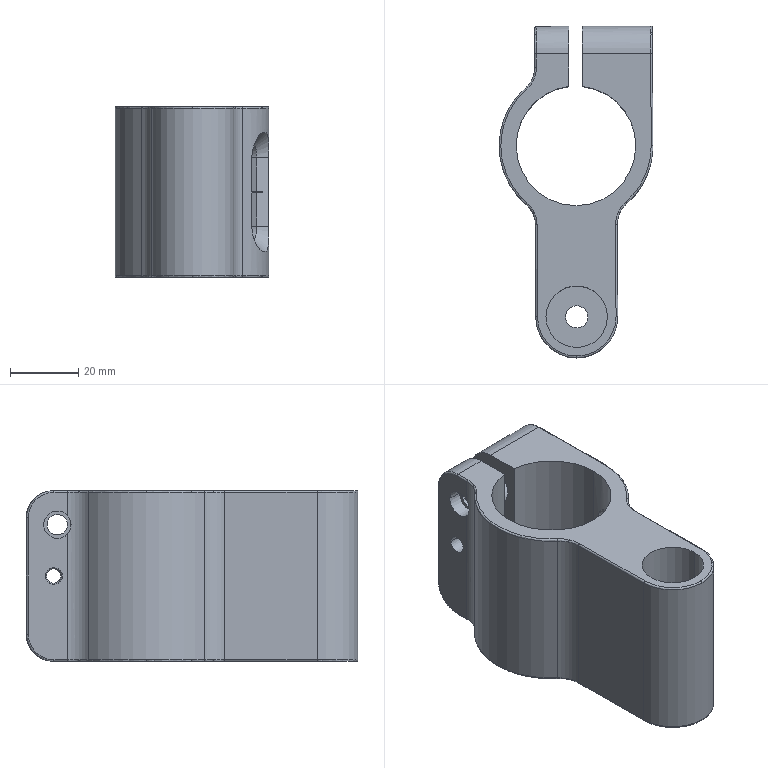Part | SolidWorks | features BaseBody 1 | 1 solid | 113 faces | box 45 x 97.095 x 50 mm | volume 87229 mm3 | cylinder 45 | spline 34 | plane 28 | cone 6 | commonest cylinder face diameters 1 x10 16 x9 8 x4 12 x4 35 x3 45 x3